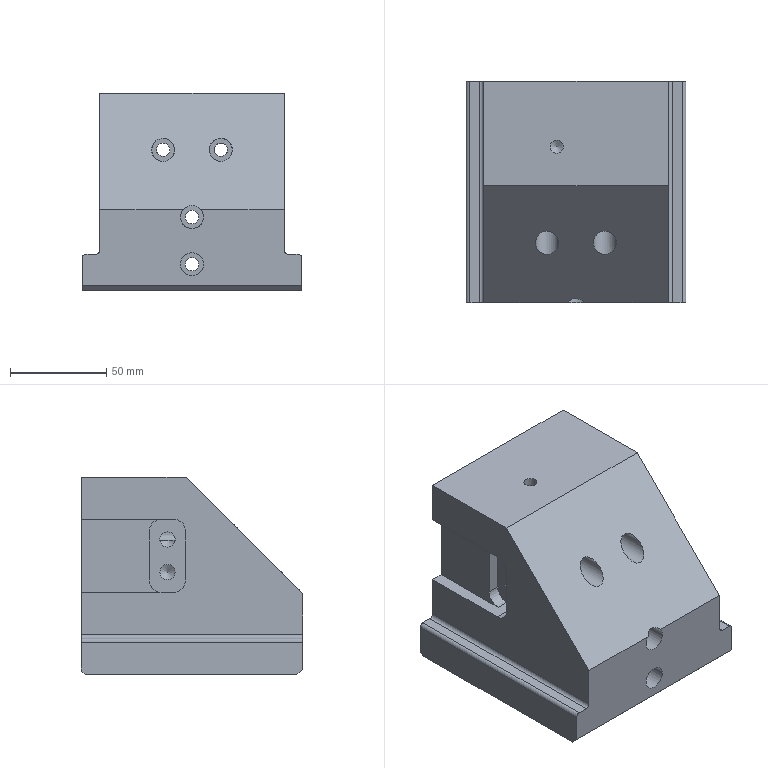Part | STEP file | 1_id834_x_t | 1 solid | 82 faces | box 114.4 x 115 x 102.9 mm | volume 813776 mm3 | plane 38 | cylinder 36 | cone 8 | commonest cylinder face diameters 13.2 x8 4 x4 6.8 x4 7 x4 7.938 x4 12 x4